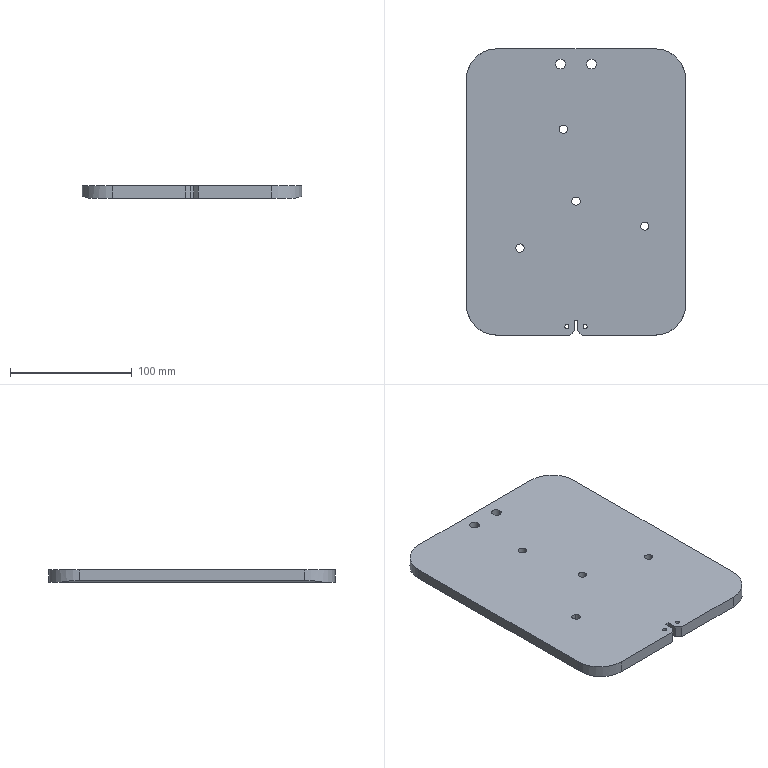Part | STEP file | Tray base | 1 solid | 34 faces | box 180 x 235 x 10 mm | volume 413174 mm3 | cylinder 20 | plane 14 | commonest cylinder face diameters 6.8 x8 3.3 x4 8 x4 50 x4